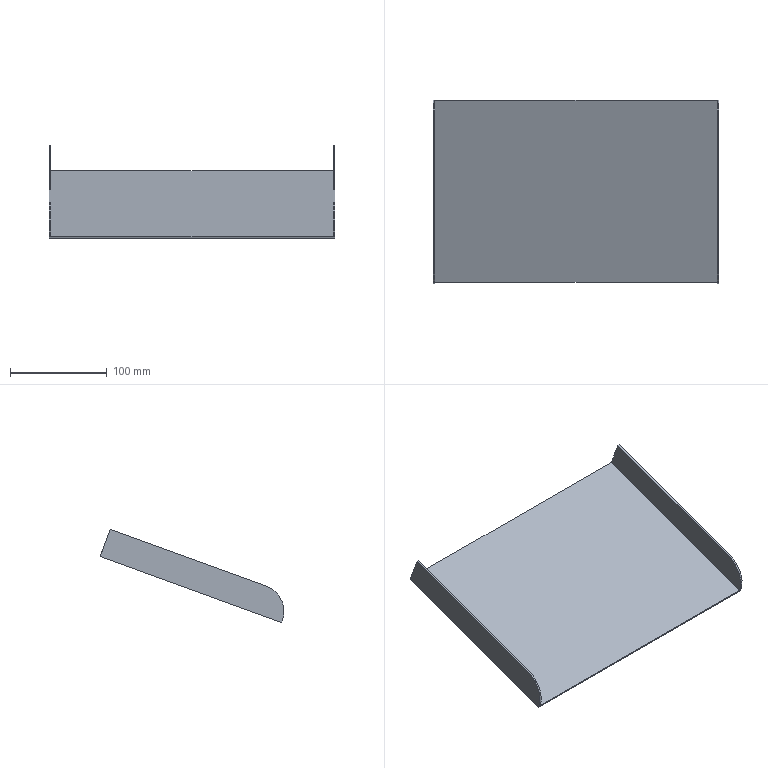Part | NX | features solid 2 | 1 solid | 12 faces | box 296.2 x 190.311 x 96.595 mm | volume 140207 mm3 | plane 10 | cylinder 2 | commonest cylinder face diameters 56 x2
STEP:
#1=CARTESIAN_POINT('',(32.,-997.939,-367.986));
#2=VERTEX_POINT('',#1);
#3=CARTESIAN_POINT('',(324.2,-997.939,-367.986));
#4=VERTEX_POINT('',#3);
#5=CARTESIAN_POINT('',(42.,-997.939,-367.986));
#6=DIRECTION('',(1.,0.,0.));
#7=VECTOR('',#6,1000.);
#8=LINE('',#5,#7);
#9=EDGE_CURVE('',#2,#4,#8,.T.);
#10=ORIENTED_EDGE('',*,*,#9,.T.);
#11=CARTESIAN_POINT('',(324.2,-810.,-299.582));
#12=VERTEX_POINT('',#11);
#13=CARTESIAN_POINT('',(324.2,-838.191,-309.843));
#14=DIRECTION('',(0.,0.9397,0.342));
#15=VECTOR('',#14,1000.);
#16=LINE('',#13,#15);
#17=EDGE_CURVE('',#4,#12,#16,.T.);
#18=ORIENTED_EDGE('',*,*,#17,.T.);
#19=CARTESIAN_POINT('',(32.,-810.,-299.582));
#20=VERTEX_POINT('',#19);
#21=CARTESIAN_POINT('',(42.,-810.,-299.582));
#22=DIRECTION('',(-1.,0.,0.));
#23=VECTOR('',#22,1000.);
#24=LINE('',#21,#23);
#25=EDGE_CURVE('',#20,#12,#24,.F.);
#26=ORIENTED_EDGE('',*,*,#25,.F.);
#27=CARTESIAN_POINT('',(32.,-838.191,-309.843));
#28=DIRECTION('',(0.,0.9397,0.342));
#29=VECTOR('',#28,1000.);
#30=LINE('',#27,#29);
#31=EDGE_CURVE('',#2,#20,#30,.T.);
#32=ORIENTED_EDGE('',*,*,#31,.F.);
#33=EDGE_LOOP('',(#10,#18,#26,#32));
#34=FACE_BOUND('',#33,.T.);
#35=CARTESIAN_POINT('',(42.,-838.191,-309.843));
#36=DIRECTION('',(0.,0.342,-0.9397));
#37=DIRECTION('',(-1.,0.,0.));
#38=AXIS2_PLACEMENT_3D('',#35,#36,#37);
#39=PLANE('',#38);
#40=ADVANCED_FACE('',(#34),#39,.F.);
#41=ORIENTED_EDGE('',*,*,#25,.T.);
#42=CARTESIAN_POINT('',(324.2,-819.577,-273.271));
#43=VERTEX_POINT('',#42);
#44=CARTESIAN_POINT('',(324.2,-809.316,-301.462));
#45=DIRECTION('',(0.,-0.342,0.9397));
#46=VECTOR('',#45,1000.);
#47=LINE('',#44,#46);
#48=EDGE_CURVE('',#12,#43,#47,.T.);
#49=ORIENTED_EDGE('',*,*,#48,.T.);
#50=CARTESIAN_POINT('',(326.2,-819.577,-273.271));
#51=VERTEX_POINT('',#50);
#52=CARTESIAN_POINT('',(326.2,-819.577,-273.271));
#53=DIRECTION('',(-1.,0.,0.));
#54=VECTOR('',#53,1000.);
#55=LINE('',#52,#54);
#56=EDGE_CURVE('',#51,#43,#55,.T.);
#57=ORIENTED_EDGE('',*,*,#56,.F.);
#58=CARTESIAN_POINT('',(326.2,-809.316,-301.462));
#59=VERTEX_POINT('',#58);
#60=CARTESIAN_POINT('',(326.2,-810.,-299.582));
#61=DIRECTION('',(0.,0.342,-0.9397));
#62=VECTOR('',#61,1000.);
#63=LINE('',#60,#62);
#64=EDGE_CURVE('',#51,#59,#63,.T.);
#65=ORIENTED_EDGE('',*,*,#64,.T.);
#66=CARTESIAN_POINT('',(30.,-809.316,-301.462));
#67=VERTEX_POINT('',#66);
#68=CARTESIAN_POINT('',(42.,-809.316,-301.462));
#69=DIRECTION('',(-1.,0.,0.));
#70=VECTOR('',#69,1000.);
#71=LINE('',#68,#70);
#72=EDGE_CURVE('',#67,#59,#71,.F.);
#73=ORIENTED_EDGE('',*,*,#72,.F.);
#74=CARTESIAN_POINT('',(30.,-819.577,-273.271));
#75=VERTEX_POINT('',#74);
#76=CARTESIAN_POINT('',(30.,-810.,-299.582));
#77=DIRECTION('',(0.,-0.342,0.9397));
#78=VECTOR('',#77,1000.);
#79=LINE('',#76,#78);
#80=EDGE_CURVE('',#75,#67,#79,.F.);
#81=ORIENTED_EDGE('',*,*,#80,.F.);
#82=CARTESIAN_POINT('',(32.,-819.577,-273.271));
#83=VERTEX_POINT('',#82);
#84=CARTESIAN_POINT('',(30.,-819.577,-273.271));
#85=DIRECTION('',(-1.,0.,0.));
#86=VECTOR('',#85,1000.);
#87=LINE('',#84,#86);
#88=EDGE_CURVE('',#75,#83,#87,.F.);
#89=ORIENTED_EDGE('',*,*,#88,.T.);
#90=CARTESIAN_POINT('',(32.,-809.316,-301.462));
#91=DIRECTION('',(0.,-0.342,0.9397));
#92=VECTOR('',#91,1000.);
#93=LINE('',#90,#92);
#94=EDGE_CURVE('',#20,#83,#93,.T.);
#95=ORIENTED_EDGE('',*,*,#94,.F.);
#96=EDGE_LOOP('',(#41,#49,#57,#65,#73,#81,#89,#95));
#97=FACE_BOUND('',#96,.T.);
#98=CARTESIAN_POINT('',(42.,-810.,-299.582));
#99=DIRECTION('',(0.,0.9397,0.342));
#100=DIRECTION('',(1.,0.,0.));
#101=AXIS2_PLACEMENT_3D('',#98,#99,#100);
#102=PLANE('',#101);
#103=ADVANCED_FACE('',(#97),#102,.T.);
#104=ORIENTED_EDGE('',*,*,#80,.T.);
#105=CARTESIAN_POINT('',(30.,-997.254,-369.866));
#106=VERTEX_POINT('',#105);
#107=CARTESIAN_POINT('',(30.,-837.507,-311.722));
#108=DIRECTION('',(0.,-0.9397,-0.342));
#109=VECTOR('',#108,1000.);
#110=LINE('',#107,#109);
#111=EDGE_CURVE('',#67,#106,#110,.T.);
#112=ORIENTED_EDGE('',*,*,#111,.T.);
#113=CARTESIAN_POINT('',(30.,-997.939,-367.986));
#114=VERTEX_POINT('',#113);
#115=CARTESIAN_POINT('',(30.,-997.939,-367.986));
#116=DIRECTION('',(0.,0.342,-0.9397));
#117=VECTOR('',#116,1000.);
#118=LINE('',#115,#117);
#119=EDGE_CURVE('',#114,#106,#118,.T.);
#120=ORIENTED_EDGE('',*,*,#119,.F.);
#121=CARTESIAN_POINT('',(30.,-981.204,-332.098));
#122=VERTEX_POINT('',#121);
#123=CARTESIAN_POINT('',(30.,-971.627,-358.41));
#124=DIRECTION('',(-1.,0.,0.));
#125=DIRECTION('',(0.,0.,1.));
#126=AXIS2_PLACEMENT_3D('',#123,#124,#125);
#127=CIRCLE('',#126,28.);
#128=EDGE_CURVE('',#114,#122,#127,.T.);
#129=ORIENTED_EDGE('',*,*,#128,.T.);
#130=CARTESIAN_POINT('',(30.,-819.577,-273.271));
#131=DIRECTION('',(0.,-0.9397,-0.342));
#132=VECTOR('',#131,1000.);
#133=LINE('',#130,#132);
#134=EDGE_CURVE('',#75,#122,#133,.T.);
#135=ORIENTED_EDGE('',*,*,#134,.F.);
#136=EDGE_LOOP('',(#104,#112,#120,#129,#135));
#137=FACE_BOUND('',#136,.T.);
#138=CARTESIAN_POINT('',(30.,-838.191,-309.843));
#139=DIRECTION('',(1.,0.,0.));
#140=DIRECTION('',(0.,-0.9397,-0.342));
#141=AXIS2_PLACEMENT_3D('',#138,#139,#140);
#142=PLANE('',#141);
#143=ADVANCED_FACE('',(#137),#142,.F.);
#144=CARTESIAN_POINT('',(326.2,-997.254,-369.866));
#145=VERTEX_POINT('',#144);
#146=CARTESIAN_POINT('',(42.,-997.254,-369.866));
#147=DIRECTION('',(-1.,0.,0.));
#148=VECTOR('',#147,1000.);
#149=LINE('',#146,#148);
#150=EDGE_CURVE('',#106,#145,#149,.F.);
#151=ORIENTED_EDGE('',*,*,#150,.T.);
#152=CARTESIAN_POINT('',(326.2,-997.939,-367.986));
#153=VERTEX_POINT('',#152);
#154=CARTESIAN_POINT('',(326.2,-997.939,-367.986));
#155=DIRECTION('',(0.,-0.342,0.9397));
#156=VECTOR('',#155,1000.);
#157=LINE('',#154,#156);
#158=EDGE_CURVE('',#153,#145,#157,.F.);
#159=ORIENTED_EDGE('',*,*,#158,.F.);
#160=CARTESIAN_POINT('',(326.2,-997.939,-367.986));
#161=DIRECTION('',(1.,0.,0.));
#162=VECTOR('',#161,1000.);
#163=LINE('',#160,#162);
#164=EDGE_CURVE('',#153,#4,#163,.F.);
#165=ORIENTED_EDGE('',*,*,#164,.T.);
#166=ORIENTED_EDGE('',*,*,#9,.F.);
#167=CARTESIAN_POINT('',(42.,-997.939,-367.986));
#168=DIRECTION('',(1.,0.,0.));
#169=VECTOR('',#168,1000.);
#170=LINE('',#167,#169);
#171=EDGE_CURVE('',#114,#2,#170,.T.);
#172=ORIENTED_EDGE('',*,*,#171,.F.);
#173=ORIENTED_EDGE('',*,*,#119,.T.);
#174=EDGE_LOOP('',(#151,#159,#165,#166,#172,#173));
#175=FACE_BOUND('',#174,.T.);
#176=CARTESIAN_POINT('',(42.,-997.939,-367.986));
#177=DIRECTION('',(0.,0.9397,0.342));
#178=DIRECTION('',(1.,0.,0.));
#179=AXIS2_PLACEMENT_3D('',#176,#177,#178);
#180=PLANE('',#179);
#181=ADVANCED_FACE('',(#175),#180,.F.);
#182=ORIENTED_EDGE('',*,*,#64,.F.);
#183=CARTESIAN_POINT('',(326.2,-981.204,-332.098));
#184=VERTEX_POINT('',#183);
#185=CARTESIAN_POINT('',(326.2,-819.577,-273.271));
#186=DIRECTION('',(0.,-0.9397,-0.342));
#187=VECTOR('',#186,1000.);
#188=LINE('',#185,#187);
#189=EDGE_CURVE('',#51,#184,#188,.T.);
#190=ORIENTED_EDGE('',*,*,#189,.T.);
#191=CARTESIAN_POINT('',(326.2,-971.627,-358.41));
#192=DIRECTION('',(-1.,0.,0.));
#193=DIRECTION('',(0.,0.,1.));
#194=AXIS2_PLACEMENT_3D('',#191,#192,#193);
#195=CIRCLE('',#194,28.);
#196=EDGE_CURVE('',#184,#153,#195,.F.);
#197=ORIENTED_EDGE('',*,*,#196,.T.);
#198=ORIENTED_EDGE('',*,*,#158,.T.);
#199=CARTESIAN_POINT('',(326.2,-837.507,-311.722));
#200=DIRECTION('',(0.,0.9397,0.342));
#201=VECTOR('',#200,1000.);
#202=LINE('',#199,#201);
#203=EDGE_CURVE('',#59,#145,#202,.F.);
#204=ORIENTED_EDGE('',*,*,#203,.F.);
#205=EDGE_LOOP('',(#182,#190,#197,#198,#204));
#206=FACE_BOUND('',#205,.T.);
#207=CARTESIAN_POINT('',(326.2,-838.191,-309.843));
#208=DIRECTION('',(1.,0.,0.));
#209=DIRECTION('',(0.,-0.9397,-0.342));
#210=AXIS2_PLACEMENT_3D('',#207,#208,#209);
#211=PLANE('',#210);
#212=ADVANCED_FACE('',(#206),#211,.T.);
#213=ORIENTED_EDGE('',*,*,#72,.T.);
#214=ORIENTED_EDGE('',*,*,#203,.T.);
#215=ORIENTED_EDGE('',*,*,#150,.F.);
#216=ORIENTED_EDGE('',*,*,#111,.F.);
#217=EDGE_LOOP('',(#213,#214,#215,#216));
#218=FACE_BOUND('',#217,.T.);
#219=CARTESIAN_POINT('',(42.,-837.507,-311.722));
#220=DIRECTION('',(0.,0.342,-0.9397));
#221=DIRECTION('',(-1.,0.,0.));
#222=AXIS2_PLACEMENT_3D('',#219,#220,#221);
#223=PLANE('',#222);
#224=ADVANCED_FACE('',(#218),#223,.T.);
#225=CARTESIAN_POINT('',(32.,-981.204,-332.098));
#226=VERTEX_POINT('',#225);
#227=CARTESIAN_POINT('',(32.,-971.627,-358.41));
#228=DIRECTION('',(-1.,0.,0.));
#229=DIRECTION('',(0.,0.,1.));
#230=AXIS2_PLACEMENT_3D('',#227,#228,#229);
#231=CIRCLE('',#230,28.);
#232=EDGE_CURVE('',#226,#2,#231,.F.);
#233=ORIENTED_EDGE('',*,*,#232,.T.);
#234=ORIENTED_EDGE('',*,*,#31,.T.);
#235=ORIENTED_EDGE('',*,*,#94,.T.);
#236=CARTESIAN_POINT('',(32.,-819.577,-273.271));
#237=DIRECTION('',(0.,0.9397,0.342));
#238=VECTOR('',#237,1000.);
#239=LINE('',#236,#238);
#240=EDGE_CURVE('',#83,#226,#239,.F.);
#241=ORIENTED_EDGE('',*,*,#240,.T.);
#242=EDGE_LOOP('',(#233,#234,#235,#241));
#243=FACE_BOUND('',#242,.T.);
#244=CARTESIAN_POINT('',(32.,-809.316,-301.462));
#245=DIRECTION('',(-1.,0.,0.));
#246=DIRECTION('',(0.,-0.342,0.9397));
#247=AXIS2_PLACEMENT_3D('',#244,#245,#246);
#248=PLANE('',#247);
#249=ADVANCED_FACE('',(#243),#248,.F.);
#250=ORIENTED_EDGE('',*,*,#134,.T.);
#251=CARTESIAN_POINT('',(30.,-981.204,-332.098));
#252=DIRECTION('',(-1.,0.,0.));
#253=VECTOR('',#252,1000.);
#254=LINE('',#251,#253);
#255=EDGE_CURVE('',#122,#226,#254,.F.);
#256=ORIENTED_EDGE('',*,*,#255,.T.);
#257=ORIENTED_EDGE('',*,*,#240,.F.);
#258=ORIENTED_EDGE('',*,*,#88,.F.);
#259=EDGE_LOOP('',(#250,#256,#257,#258));
#260=FACE_BOUND('',#259,.T.);
#261=CARTESIAN_POINT('',(30.,-819.577,-273.271));
#262=DIRECTION('',(0.,0.342,-0.9397));
#263=DIRECTION('',(0.,-0.9397,-0.342));
#264=AXIS2_PLACEMENT_3D('',#261,#262,#263);
#265=PLANE('',#264);
#266=ADVANCED_FACE('',(#260),#265,.F.);
#267=ORIENTED_EDGE('',*,*,#128,.F.);
#268=ORIENTED_EDGE('',*,*,#171,.T.);
#269=ORIENTED_EDGE('',*,*,#232,.F.);
#270=ORIENTED_EDGE('',*,*,#255,.F.);
#271=EDGE_LOOP('',(#267,#268,#269,#270));
#272=FACE_BOUND('',#271,.T.);
#273=CARTESIAN_POINT('',(30.,-971.627,-358.41));
#274=DIRECTION('',(-1.,0.,0.));
#275=DIRECTION('',(0.,0.,1.));
#276=AXIS2_PLACEMENT_3D('',#273,#274,#275);
#277=CYLINDRICAL_SURFACE('',#276,28.);
#278=ADVANCED_FACE('',(#272),#277,.T.);
#279=ORIENTED_EDGE('',*,*,#17,.F.);
#280=CARTESIAN_POINT('',(324.2,-981.204,-332.098));
#281=VERTEX_POINT('',#280);
#282=CARTESIAN_POINT('',(324.2,-971.627,-358.41));
#283=DIRECTION('',(-1.,0.,0.));
#284=DIRECTION('',(0.,0.,1.));
#285=AXIS2_PLACEMENT_3D('',#282,#283,#284);
#286=CIRCLE('',#285,28.);
#287=EDGE_CURVE('',#4,#281,#286,.T.);
#288=ORIENTED_EDGE('',*,*,#287,.T.);
#289=CARTESIAN_POINT('',(324.2,-819.577,-273.271));
#290=DIRECTION('',(0.,0.9397,0.342));
#291=VECTOR('',#290,1000.);
#292=LINE('',#289,#291);
#293=EDGE_CURVE('',#43,#281,#292,.F.);
#294=ORIENTED_EDGE('',*,*,#293,.F.);
#295=ORIENTED_EDGE('',*,*,#48,.F.);
#296=EDGE_LOOP('',(#279,#288,#294,#295));
#297=FACE_BOUND('',#296,.T.);
#298=CARTESIAN_POINT('',(324.2,-809.316,-301.462));
#299=DIRECTION('',(-1.,0.,0.));
#300=DIRECTION('',(0.,-0.342,0.9397));
#301=AXIS2_PLACEMENT_3D('',#298,#299,#300);
#302=PLANE('',#301);
#303=ADVANCED_FACE('',(#297),#302,.T.);
#304=ORIENTED_EDGE('',*,*,#293,.T.);
#305=CARTESIAN_POINT('',(326.2,-981.204,-332.098));
#306=DIRECTION('',(-1.,0.,0.));
#307=VECTOR('',#306,1000.);
#308=LINE('',#305,#307);
#309=EDGE_CURVE('',#281,#184,#308,.F.);
#310=ORIENTED_EDGE('',*,*,#309,.T.);
#311=ORIENTED_EDGE('',*,*,#189,.F.);
#312=ORIENTED_EDGE('',*,*,#56,.T.);
#313=EDGE_LOOP('',(#304,#310,#311,#312));
#314=FACE_BOUND('',#313,.T.);
#315=CARTESIAN_POINT('',(326.2,-819.577,-273.271));
#316=DIRECTION('',(0.,0.342,-0.9397));
#317=DIRECTION('',(0.,-0.9397,-0.342));
#318=AXIS2_PLACEMENT_3D('',#315,#316,#317);
#319=PLANE('',#318);
#320=ADVANCED_FACE('',(#314),#319,.F.);
#321=ORIENTED_EDGE('',*,*,#196,.F.);
#322=ORIENTED_EDGE('',*,*,#309,.F.);
#323=ORIENTED_EDGE('',*,*,#287,.F.);
#324=ORIENTED_EDGE('',*,*,#164,.F.);
#325=EDGE_LOOP('',(#321,#322,#323,#324));
#326=FACE_BOUND('',#325,.T.);
#327=CARTESIAN_POINT('',(326.2,-971.627,-358.41));
#328=DIRECTION('',(1.,0.,0.));
#329=DIRECTION('',(0.,0.,-1.));
#330=AXIS2_PLACEMENT_3D('',#327,#328,#329);
#331=CYLINDRICAL_SURFACE('',#330,28.);
#332=ADVANCED_FACE('',(#326),#331,.T.);
#333=CLOSED_SHELL('',(#40,#103,#143,#181,#212,#224,#249,#266,#278,#303,#320,#332));
#334=MANIFOLD_SOLID_BREP('',#333);
#335=(LENGTH_UNIT()NAMED_UNIT(*)SI_UNIT(.MILLI.,.METRE.));
#336=UNCERTAINTY_MEASURE_WITH_UNIT(LENGTH_MEASURE(0.00001),#335,'','');
#337=(NAMED_UNIT(*)PLANE_ANGLE_UNIT()SI_UNIT($,.RADIAN.));
#338=(NAMED_UNIT(*)SI_UNIT($,.STERADIAN.)SOLID_ANGLE_UNIT());
#339=(GEOMETRIC_REPRESENTATION_CONTEXT(3)GLOBAL_UNCERTAINTY_ASSIGNED_CONTEXT((#336))GLOBAL_UNIT_ASSIGNED_CONTEXT((#335,#337,#338))REPRESENTATION_CONTEXT('',''));
#340=ADVANCED_BREP_SHAPE_REPRESENTATION('',(#334),#339);